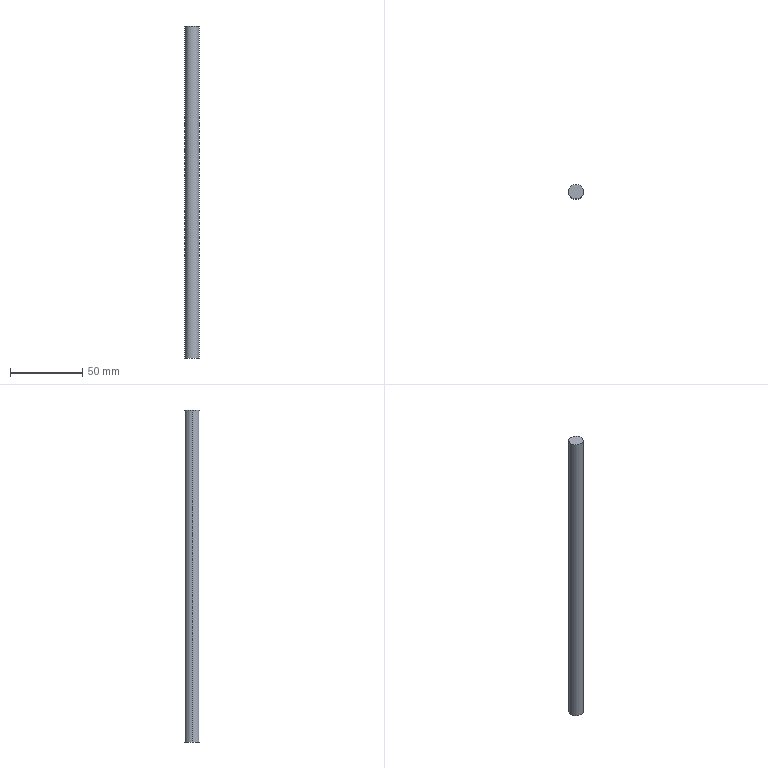Part | SolidWorks | features BaseBody 1 | 1 solid | 4 faces | box 10 x 10 x 230 mm | volume 18064 mm3 | cylinder 2 | plane 2 | commonest cylinder face diameters 10 x2
STEP:
#1=CARTESIAN_POINT('',(884.019,-3537.473,580.189));
#2=VERTEX_POINT('',#1);
#3=CARTESIAN_POINT('',(874.019,-3537.473,580.189));
#4=VERTEX_POINT('',#3);
#5=CARTESIAN_POINT('',(879.019,-3537.473,580.189));
#6=DIRECTION('',(0.,0.,1.));
#7=DIRECTION('',(1.,0.,0.));
#8=AXIS2_PLACEMENT_3D('',#5,#6,#7);
#9=CIRCLE('',#8,5.);
#10=EDGE_CURVE('',#2,#4,#9,.T.);
#11=ORIENTED_EDGE('',*,*,#10,.T.);
#12=CARTESIAN_POINT('',(874.019,-3537.473,810.189));
#13=VERTEX_POINT('',#12);
#14=CARTESIAN_POINT('',(874.019,-3537.473,680.189));
#15=DIRECTION('',(0.,0.,1.));
#16=VECTOR('',#15,1000.);
#17=LINE('',#14,#16);
#18=EDGE_CURVE('',#4,#13,#17,.T.);
#19=ORIENTED_EDGE('',*,*,#18,.T.);
#20=CARTESIAN_POINT('',(884.019,-3537.473,810.189));
#21=VERTEX_POINT('',#20);
#22=CARTESIAN_POINT('',(879.019,-3537.473,810.189));
#23=DIRECTION('',(0.,0.,-1.));
#24=DIRECTION('',(1.,0.,0.));
#25=AXIS2_PLACEMENT_3D('',#22,#23,#24);
#26=CIRCLE('',#25,5.);
#27=EDGE_CURVE('',#13,#21,#26,.T.);
#28=ORIENTED_EDGE('',*,*,#27,.T.);
#29=CARTESIAN_POINT('',(884.019,-3537.473,680.189));
#30=DIRECTION('',(0.,0.,1.));
#31=VECTOR('',#30,1000.);
#32=LINE('',#29,#31);
#33=EDGE_CURVE('',#2,#21,#32,.T.);
#34=ORIENTED_EDGE('',*,*,#33,.F.);
#35=EDGE_LOOP('',(#11,#19,#28,#34));
#36=FACE_OUTER_BOUND('',#35,.T.);
#37=CARTESIAN_POINT('',(879.019,-3537.473,680.189));
#38=DIRECTION('',(0.,0.,1.));
#39=DIRECTION('',(1.,0.,0.));
#40=AXIS2_PLACEMENT_3D('',#37,#38,#39);
#41=CYLINDRICAL_SURFACE('',#40,5.);
#42=ADVANCED_FACE('',(#36),#41,.T.);
#43=ORIENTED_EDGE('',*,*,#18,.F.);
#44=CARTESIAN_POINT('',(879.019,-3537.473,580.189));
#45=DIRECTION('',(0.,0.,1.));
#46=DIRECTION('',(1.,0.,0.));
#47=AXIS2_PLACEMENT_3D('',#44,#45,#46);
#48=CIRCLE('',#47,5.);
#49=EDGE_CURVE('',#4,#2,#48,.T.);
#50=ORIENTED_EDGE('',*,*,#49,.T.);
#51=ORIENTED_EDGE('',*,*,#33,.T.);
#52=CARTESIAN_POINT('',(879.019,-3537.473,810.189));
#53=DIRECTION('',(0.,0.,-1.));
#54=DIRECTION('',(1.,0.,0.));
#55=AXIS2_PLACEMENT_3D('',#52,#53,#54);
#56=CIRCLE('',#55,5.);
#57=EDGE_CURVE('',#21,#13,#56,.T.);
#58=ORIENTED_EDGE('',*,*,#57,.T.);
#59=EDGE_LOOP('',(#43,#50,#51,#58));
#60=FACE_OUTER_BOUND('',#59,.T.);
#61=CARTESIAN_POINT('',(879.019,-3537.473,680.189));
#62=DIRECTION('',(0.,0.,1.));
#63=DIRECTION('',(1.,0.,0.));
#64=AXIS2_PLACEMENT_3D('',#61,#62,#63);
#65=CYLINDRICAL_SURFACE('',#64,5.);
#66=ADVANCED_FACE('',(#60),#65,.T.);
#67=ORIENTED_EDGE('',*,*,#57,.F.);
#68=ORIENTED_EDGE('',*,*,#27,.F.);
#69=EDGE_LOOP('',(#67,#68));
#70=FACE_OUTER_BOUND('',#69,.T.);
#71=CARTESIAN_POINT('',(879.019,-3537.473,810.189));
#72=DIRECTION('',(0.,0.,1.));
#73=DIRECTION('',(1.,0.,0.));
#74=AXIS2_PLACEMENT_3D('',#71,#72,#73);
#75=PLANE('',#74);
#76=ADVANCED_FACE('',(#70),#75,.T.);
#77=ORIENTED_EDGE('',*,*,#10,.F.);
#78=ORIENTED_EDGE('',*,*,#49,.F.);
#79=EDGE_LOOP('',(#77,#78));
#80=FACE_OUTER_BOUND('',#79,.T.);
#81=CARTESIAN_POINT('',(879.019,-3537.473,580.189));
#82=DIRECTION('',(0.,0.,-1.));
#83=DIRECTION('',(-1.,0.,0.));
#84=AXIS2_PLACEMENT_3D('',#81,#82,#83);
#85=PLANE('',#84);
#86=ADVANCED_FACE('',(#80),#85,.T.);
#87=CLOSED_SHELL('',(#42,#66,#76,#86));
#88=MANIFOLD_SOLID_BREP('',#87);
#89=CARTESIAN_POINT('',(0.,0.,0.));
#90=DIRECTION('',(0.,0.,1.));
#91=DIRECTION('',(1.,0.,0.));
#92=AXIS2_PLACEMENT_3D('',#89,#90,#91);
#93=(LENGTH_UNIT()NAMED_UNIT(*)SI_UNIT(.MILLI.,.METRE.));
#94=UNCERTAINTY_MEASURE_WITH_UNIT(LENGTH_MEASURE(0.00001),#93,'','');
#95=(NAMED_UNIT(*)PLANE_ANGLE_UNIT()SI_UNIT($,.RADIAN.));
#96=(NAMED_UNIT(*)SI_UNIT($,.STERADIAN.)SOLID_ANGLE_UNIT());
#97=(GEOMETRIC_REPRESENTATION_CONTEXT(3)GLOBAL_UNCERTAINTY_ASSIGNED_CONTEXT((#94))GLOBAL_UNIT_ASSIGNED_CONTEXT((#93,#95,#96))REPRESENTATION_CONTEXT('',''));
#98=ADVANCED_BREP_SHAPE_REPRESENTATION('',(#88,#92),#97);